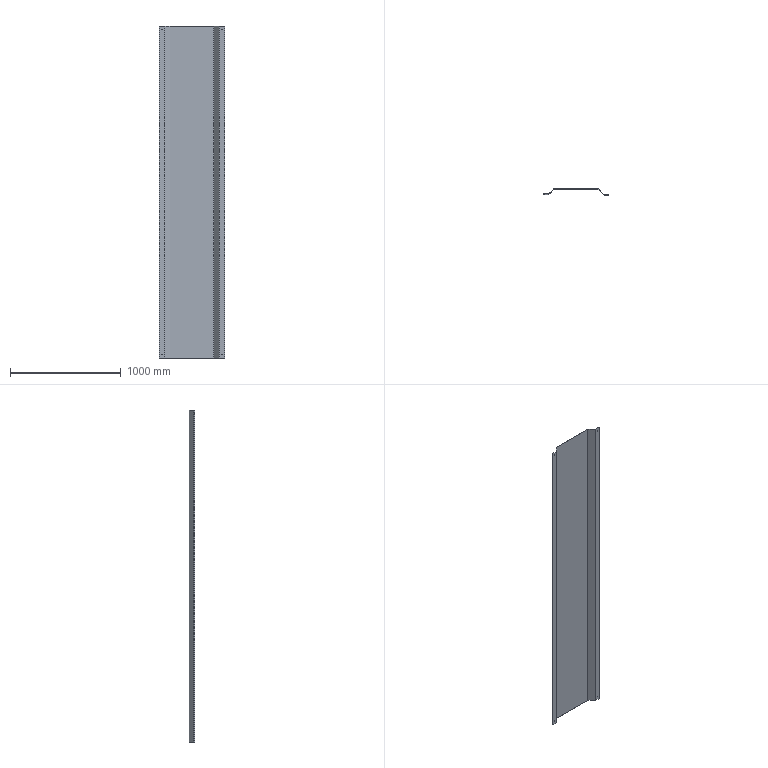Part | STEP file | Assembly TS-S01 | 1 solid | 46 faces | box 590.109 x 52.135 x 2995 mm | volume 3761784 mm3 | plane 30 | cylinder 16 | commonest cylinder face diameters 5 x8 0.4 x4 4.4 x4